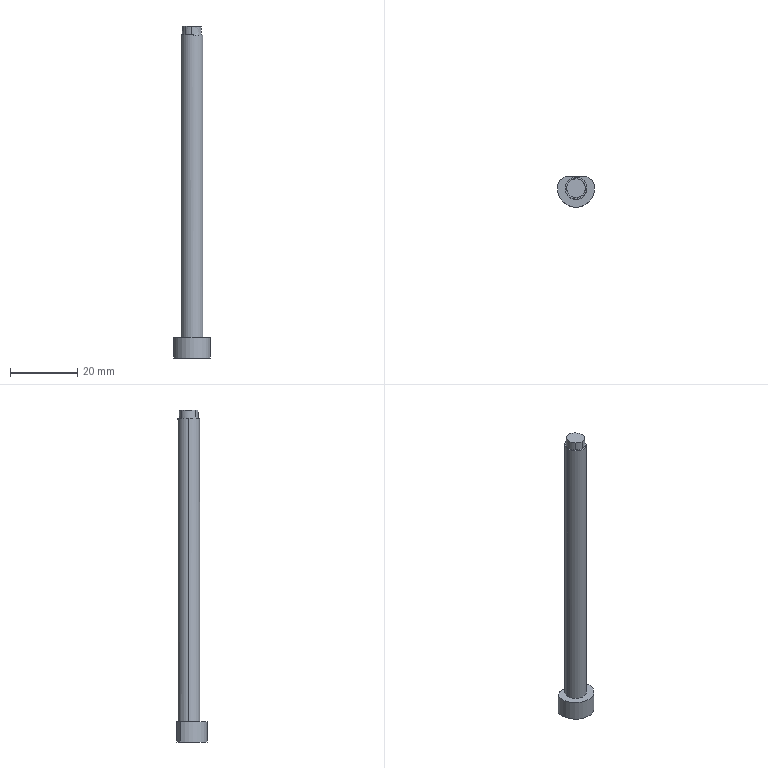Part | Creo | 1 solid | 59 faces | box 11 x 8.992 x 98.783 mm | volume 3545 mm3 | other 30 | plane 22 | cylinder 4 | spline 3 | commonest cylinder face diameters 6.5 x2 5.497 x1 11 x1